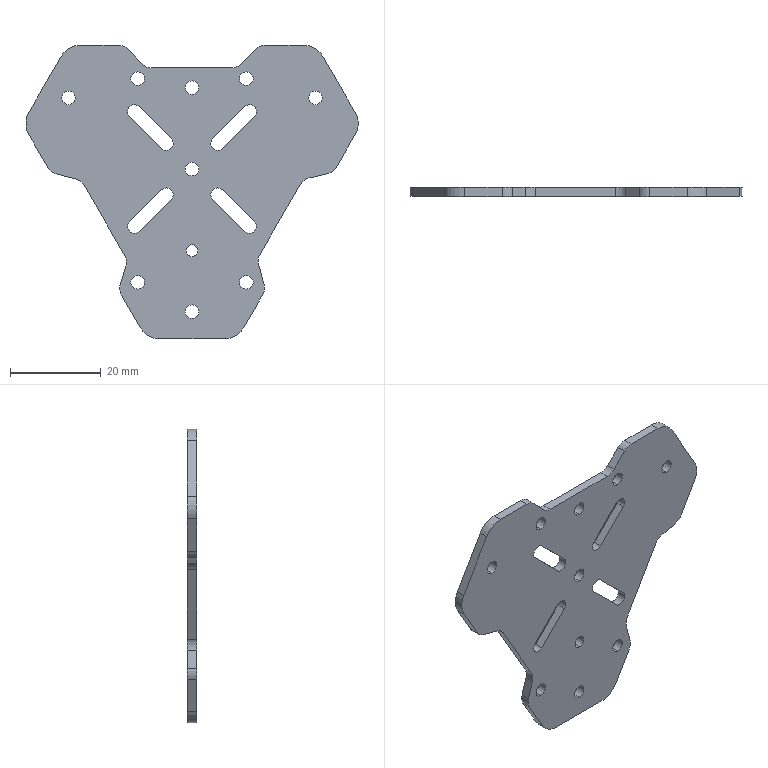Part | SolidWorks | features BaseBody 1 | 1 solid | 78 faces | box 73.405 x 2 x 64.91 mm | volume 5563 mm3 | cylinder 50 | plane 28 | commonest cylinder face diameters 3 x30 6 x12 10 x6 2.64 x2